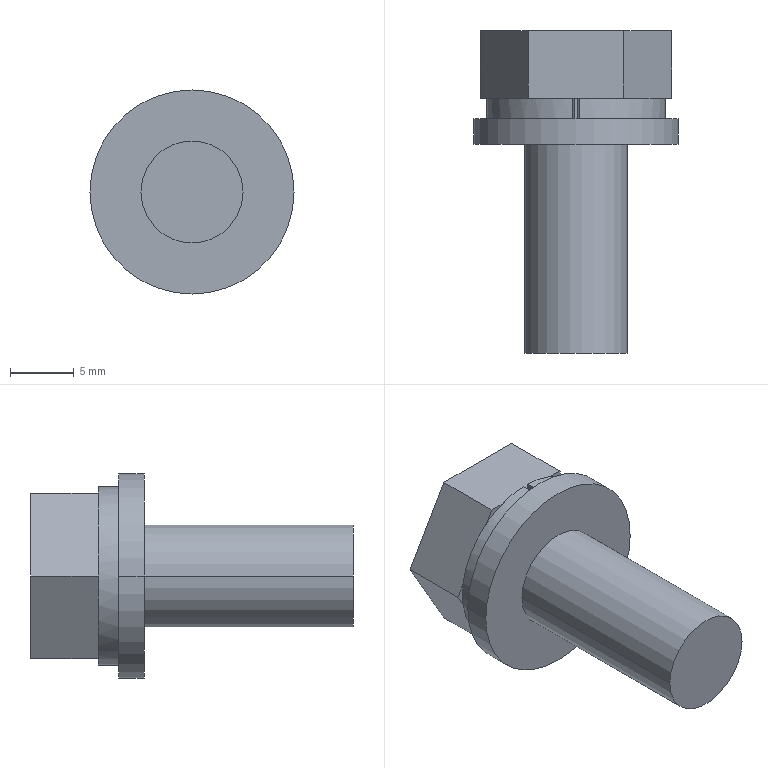Part | STEP file | LIB_36623161_M8X20 | 1 solid | 32 faces | box 16 x 25.3 x 16 mm | volume 2247 mm3 | plane 26 | cylinder 6 | commonest cylinder face diameters 8 x3 16 x2 14 x1